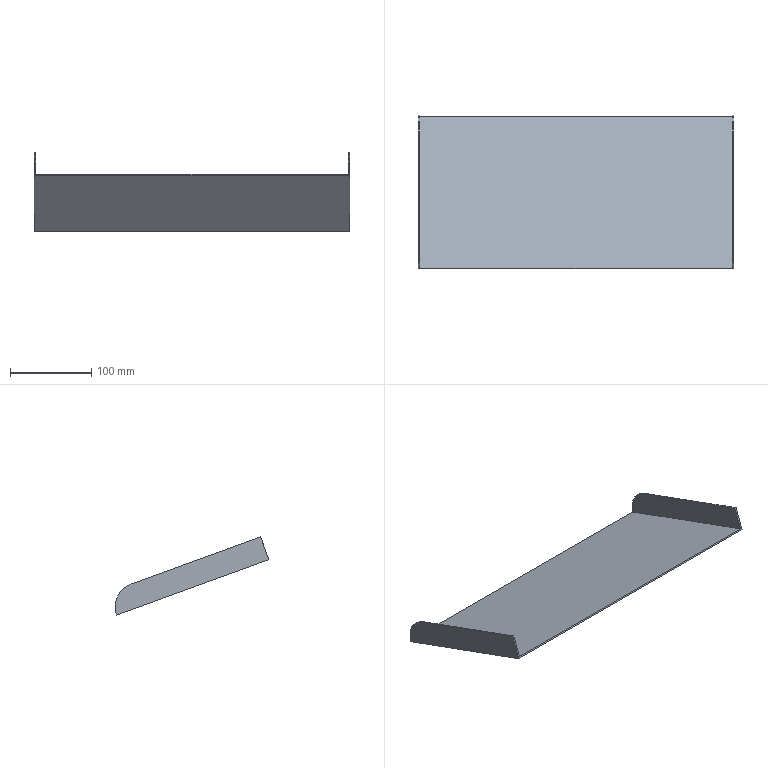Part | NX | features solid 2 | 1 solid | 12 faces | box 389.78 x 189.748 x 96.595 mm | volume 177540 mm3 | plane 10 | cylinder 2 | commonest cylinder face diameters 60 x2
STEP:
#1=CARTESIAN_POINT('',(397.22,1010.,-315.103));
#2=VERTEX_POINT('',#1);
#3=CARTESIAN_POINT('',(397.22,1197.876,-383.484));
#4=VERTEX_POINT('',#3);
#5=CARTESIAN_POINT('',(397.22,1038.191,-325.364));
#6=DIRECTION('',(0.,0.9397,-0.342));
#7=VECTOR('',#6,1000.);
#8=LINE('',#5,#7);
#9=EDGE_CURVE('',#2,#4,#8,.T.);
#10=ORIENTED_EDGE('',*,*,#9,.F.);
#11=CARTESIAN_POINT('',(783.,1010.,-315.103));
#12=VERTEX_POINT('',#11);
#13=CARTESIAN_POINT('',(407.22,1010.,-315.103));
#14=DIRECTION('',(-1.,0.,0.));
#15=VECTOR('',#14,1000.);
#16=LINE('',#13,#15);
#17=EDGE_CURVE('',#2,#12,#16,.F.);
#18=ORIENTED_EDGE('',*,*,#17,.T.);
#19=CARTESIAN_POINT('',(783.,1197.876,-383.484));
#20=VERTEX_POINT('',#19);
#21=CARTESIAN_POINT('',(783.,1038.191,-325.364));
#22=DIRECTION('',(0.,0.9397,-0.342));
#23=VECTOR('',#22,1000.);
#24=LINE('',#21,#23);
#25=EDGE_CURVE('',#12,#20,#24,.T.);
#26=ORIENTED_EDGE('',*,*,#25,.T.);
#27=CARTESIAN_POINT('',(785.,1197.876,-383.484));
#28=VERTEX_POINT('',#27);
#29=CARTESIAN_POINT('',(785.,1197.876,-383.484));
#30=CARTESIAN_POINT('',(784.333,1197.876,-383.484));
#31=CARTESIAN_POINT('',(783.667,1197.876,-383.484));
#32=CARTESIAN_POINT('',(783.,1197.876,-383.484));
#33=B_SPLINE_CURVE_WITH_KNOTS('',3,(#29,#30,#31,#32),.UNSPECIFIED.,.F.,.F.,(4,4),(1310.699,1310.701),.UNSPECIFIED.);
#34=EDGE_CURVE('',#28,#20,#33,.T.);
#35=ORIENTED_EDGE('',*,*,#34,.F.);
#36=CARTESIAN_POINT('',(785.,1197.939,-383.507));
#37=VERTEX_POINT('',#36);
#38=CARTESIAN_POINT('',(785.,1038.191,-325.364));
#39=DIRECTION('',(0.,-0.9397,0.342));
#40=VECTOR('',#39,1000.);
#41=LINE('',#38,#40);
#42=EDGE_CURVE('',#28,#37,#41,.F.);
#43=ORIENTED_EDGE('',*,*,#42,.T.);
#44=CARTESIAN_POINT('',(395.22,1197.939,-383.507));
#45=VERTEX_POINT('',#44);
#46=CARTESIAN_POINT('',(407.22,1197.939,-383.507));
#47=DIRECTION('',(1.,0.,0.));
#48=VECTOR('',#47,1000.);
#49=LINE('',#46,#48);
#50=EDGE_CURVE('',#45,#37,#49,.T.);
#51=ORIENTED_EDGE('',*,*,#50,.F.);
#52=CARTESIAN_POINT('',(395.22,1197.876,-383.484));
#53=VERTEX_POINT('',#52);
#54=CARTESIAN_POINT('',(395.22,1038.191,-325.364));
#55=DIRECTION('',(0.,0.9397,-0.342));
#56=VECTOR('',#55,1000.);
#57=LINE('',#54,#56);
#58=EDGE_CURVE('',#53,#45,#57,.T.);
#59=ORIENTED_EDGE('',*,*,#58,.F.);
#60=CARTESIAN_POINT('',(397.22,1197.876,-383.484));
#61=CARTESIAN_POINT('',(396.553,1197.876,-383.484));
#62=CARTESIAN_POINT('',(395.886,1197.876,-383.484));
#63=CARTESIAN_POINT('',(395.22,1197.876,-383.484));
#64=B_SPLINE_CURVE_WITH_KNOTS('',3,(#60,#61,#62,#63),.UNSPECIFIED.,.F.,.F.,(4,4),(1310.699,1310.701),.UNSPECIFIED.);
#65=EDGE_CURVE('',#4,#53,#64,.T.);
#66=ORIENTED_EDGE('',*,*,#65,.F.);
#67=EDGE_LOOP('',(#10,#18,#26,#35,#43,#51,#59,#66));
#68=FACE_BOUND('',#67,.T.);
#69=CARTESIAN_POINT('',(407.22,1038.191,-325.364));
#70=DIRECTION('',(0.,0.342,0.9397));
#71=DIRECTION('',(1.,0.,0.));
#72=AXIS2_PLACEMENT_3D('',#69,#70,#71);
#73=PLANE('',#72);
#74=ADVANCED_FACE('',(#68),#73,.T.);
#75=ORIENTED_EDGE('',*,*,#17,.F.);
#76=CARTESIAN_POINT('',(397.22,1019.577,-288.792));
#77=VERTEX_POINT('',#76);
#78=CARTESIAN_POINT('',(397.22,1009.316,-316.982));
#79=DIRECTION('',(0.,-0.342,-0.9397));
#80=VECTOR('',#79,1000.);
#81=LINE('',#78,#80);
#82=EDGE_CURVE('',#2,#77,#81,.F.);
#83=ORIENTED_EDGE('',*,*,#82,.T.);
#84=CARTESIAN_POINT('',(395.22,1019.577,-288.792));
#85=VERTEX_POINT('',#84);
#86=CARTESIAN_POINT('',(395.22,1019.577,-288.792));
#87=DIRECTION('',(1.,0.,0.));
#88=VECTOR('',#87,1000.);
#89=LINE('',#86,#88);
#90=EDGE_CURVE('',#85,#77,#89,.T.);
#91=ORIENTED_EDGE('',*,*,#90,.F.);
#92=CARTESIAN_POINT('',(395.22,1009.316,-316.982));
#93=VERTEX_POINT('',#92);
#94=CARTESIAN_POINT('',(395.22,1010.,-315.103));
#95=DIRECTION('',(0.,0.342,0.9397));
#96=VECTOR('',#95,1000.);
#97=LINE('',#94,#96);
#98=EDGE_CURVE('',#85,#93,#97,.F.);
#99=ORIENTED_EDGE('',*,*,#98,.T.);
#100=CARTESIAN_POINT('',(785.,1009.316,-316.982));
#101=VERTEX_POINT('',#100);
#102=CARTESIAN_POINT('',(407.22,1009.316,-316.982));
#103=DIRECTION('',(-1.,0.,0.));
#104=VECTOR('',#103,1000.);
#105=LINE('',#102,#104);
#106=EDGE_CURVE('',#93,#101,#105,.F.);
#107=ORIENTED_EDGE('',*,*,#106,.T.);
#108=CARTESIAN_POINT('',(785.,1019.577,-288.792));
#109=VERTEX_POINT('',#108);
#110=CARTESIAN_POINT('',(785.,1010.,-315.103));
#111=DIRECTION('',(0.,-0.342,-0.9397));
#112=VECTOR('',#111,1000.);
#113=LINE('',#110,#112);
#114=EDGE_CURVE('',#109,#101,#113,.T.);
#115=ORIENTED_EDGE('',*,*,#114,.F.);
#116=CARTESIAN_POINT('',(783.,1019.577,-288.792));
#117=VERTEX_POINT('',#116);
#118=CARTESIAN_POINT('',(785.,1019.577,-288.792));
#119=DIRECTION('',(1.,0.,0.));
#120=VECTOR('',#119,1000.);
#121=LINE('',#118,#120);
#122=EDGE_CURVE('',#109,#117,#121,.F.);
#123=ORIENTED_EDGE('',*,*,#122,.T.);
#124=CARTESIAN_POINT('',(783.,1009.316,-316.982));
#125=DIRECTION('',(0.,-0.342,-0.9397));
#126=VECTOR('',#125,1000.);
#127=LINE('',#124,#126);
#128=EDGE_CURVE('',#12,#117,#127,.F.);
#129=ORIENTED_EDGE('',*,*,#128,.F.);
#130=EDGE_LOOP('',(#75,#83,#91,#99,#107,#115,#123,#129));
#131=FACE_BOUND('',#130,.T.);
#132=CARTESIAN_POINT('',(407.22,1010.,-315.103));
#133=DIRECTION('',(0.,-0.9397,0.342));
#134=DIRECTION('',(1.,0.,0.));
#135=AXIS2_PLACEMENT_3D('',#132,#133,#134);
#136=PLANE('',#135);
#137=ADVANCED_FACE('',(#131),#136,.T.);
#138=ORIENTED_EDGE('',*,*,#42,.F.);
#139=CARTESIAN_POINT('',(785.,1179.324,-346.935));
#140=VERTEX_POINT('',#139);
#141=CARTESIAN_POINT('',(785.,1169.064,-375.126));
#142=DIRECTION('',(1.,0.,0.));
#143=DIRECTION('',(0.,-0.342,-0.9397));
#144=AXIS2_PLACEMENT_3D('',#141,#142,#143);
#145=CIRCLE('',#144,30.);
#146=EDGE_CURVE('',#28,#140,#145,.T.);
#147=ORIENTED_EDGE('',*,*,#146,.T.);
#148=CARTESIAN_POINT('',(785.,1019.577,-288.792));
#149=DIRECTION('',(0.,0.9397,-0.342));
#150=VECTOR('',#149,1000.);
#151=LINE('',#148,#150);
#152=EDGE_CURVE('',#109,#140,#151,.T.);
#153=ORIENTED_EDGE('',*,*,#152,.F.);
#154=ORIENTED_EDGE('',*,*,#114,.T.);
#155=CARTESIAN_POINT('',(785.,1197.254,-385.386));
#156=VERTEX_POINT('',#155);
#157=CARTESIAN_POINT('',(785.,1037.507,-327.243));
#158=DIRECTION('',(0.,-0.9397,0.342));
#159=VECTOR('',#158,1000.);
#160=LINE('',#157,#159);
#161=EDGE_CURVE('',#101,#156,#160,.F.);
#162=ORIENTED_EDGE('',*,*,#161,.T.);
#163=CARTESIAN_POINT('',(785.,1197.939,-383.507));
#164=DIRECTION('',(0.,0.342,0.9397));
#165=VECTOR('',#164,1000.);
#166=LINE('',#163,#165);
#167=EDGE_CURVE('',#37,#156,#166,.F.);
#168=ORIENTED_EDGE('',*,*,#167,.F.);
#169=EDGE_LOOP('',(#138,#147,#153,#154,#162,#168));
#170=FACE_BOUND('',#169,.T.);
#171=CARTESIAN_POINT('',(785.,1038.191,-325.364));
#172=DIRECTION('',(1.,0.,0.));
#173=DIRECTION('',(0.,0.9397,-0.342));
#174=AXIS2_PLACEMENT_3D('',#171,#172,#173);
#175=PLANE('',#174);
#176=ADVANCED_FACE('',(#170),#175,.T.);
#177=ORIENTED_EDGE('',*,*,#167,.T.);
#178=CARTESIAN_POINT('',(395.22,1197.254,-385.386));
#179=VERTEX_POINT('',#178);
#180=CARTESIAN_POINT('',(407.22,1197.254,-385.386));
#181=DIRECTION('',(1.,0.,0.));
#182=VECTOR('',#181,1000.);
#183=LINE('',#180,#182);
#184=EDGE_CURVE('',#179,#156,#183,.T.);
#185=ORIENTED_EDGE('',*,*,#184,.F.);
#186=CARTESIAN_POINT('',(395.22,1197.939,-383.507));
#187=DIRECTION('',(0.,-0.342,-0.9397));
#188=VECTOR('',#187,1000.);
#189=LINE('',#186,#188);
#190=EDGE_CURVE('',#45,#179,#189,.T.);
#191=ORIENTED_EDGE('',*,*,#190,.F.);
#192=ORIENTED_EDGE('',*,*,#50,.T.);
#193=EDGE_LOOP('',(#177,#185,#191,#192));
#194=FACE_BOUND('',#193,.T.);
#195=CARTESIAN_POINT('',(407.22,1197.939,-383.507));
#196=DIRECTION('',(0.,-0.9397,0.342));
#197=DIRECTION('',(1.,0.,0.));
#198=AXIS2_PLACEMENT_3D('',#195,#196,#197);
#199=PLANE('',#198);
#200=ADVANCED_FACE('',(#194),#199,.F.);
#201=ORIENTED_EDGE('',*,*,#190,.T.);
#202=CARTESIAN_POINT('',(395.22,1037.507,-327.243));
#203=DIRECTION('',(0.,0.9397,-0.342));
#204=VECTOR('',#203,1000.);
#205=LINE('',#202,#204);
#206=EDGE_CURVE('',#93,#179,#205,.T.);
#207=ORIENTED_EDGE('',*,*,#206,.F.);
#208=ORIENTED_EDGE('',*,*,#98,.F.);
#209=CARTESIAN_POINT('',(395.22,1179.324,-346.935));
#210=VERTEX_POINT('',#209);
#211=CARTESIAN_POINT('',(395.22,1019.577,-288.792));
#212=DIRECTION('',(0.,0.9397,-0.342));
#213=VECTOR('',#212,1000.);
#214=LINE('',#211,#213);
#215=EDGE_CURVE('',#85,#210,#214,.T.);
#216=ORIENTED_EDGE('',*,*,#215,.T.);
#217=CARTESIAN_POINT('',(395.22,1169.064,-375.126));
#218=DIRECTION('',(1.,0.,0.));
#219=DIRECTION('',(0.,-0.342,-0.9397));
#220=AXIS2_PLACEMENT_3D('',#217,#218,#219);
#221=CIRCLE('',#220,30.);
#222=EDGE_CURVE('',#210,#53,#221,.F.);
#223=ORIENTED_EDGE('',*,*,#222,.T.);
#224=ORIENTED_EDGE('',*,*,#58,.T.);
#225=EDGE_LOOP('',(#201,#207,#208,#216,#223,#224));
#226=FACE_BOUND('',#225,.T.);
#227=CARTESIAN_POINT('',(395.22,1038.191,-325.364));
#228=DIRECTION('',(1.,0.,0.));
#229=DIRECTION('',(0.,0.9397,-0.342));
#230=AXIS2_PLACEMENT_3D('',#227,#228,#229);
#231=PLANE('',#230);
#232=ADVANCED_FACE('',(#226),#231,.F.);
#233=ORIENTED_EDGE('',*,*,#161,.F.);
#234=ORIENTED_EDGE('',*,*,#106,.F.);
#235=ORIENTED_EDGE('',*,*,#206,.T.);
#236=ORIENTED_EDGE('',*,*,#184,.T.);
#237=EDGE_LOOP('',(#233,#234,#235,#236));
#238=FACE_BOUND('',#237,.T.);
#239=CARTESIAN_POINT('',(407.22,1037.507,-327.243));
#240=DIRECTION('',(0.,0.342,0.9397));
#241=DIRECTION('',(1.,0.,0.));
#242=AXIS2_PLACEMENT_3D('',#239,#240,#241);
#243=PLANE('',#242);
#244=ADVANCED_FACE('',(#238),#243,.F.);
#245=ORIENTED_EDGE('',*,*,#152,.T.);
#246=CARTESIAN_POINT('',(783.,1179.324,-346.935));
#247=VERTEX_POINT('',#246);
#248=CARTESIAN_POINT('',(785.,1179.324,-346.935));
#249=DIRECTION('',(1.,0.,0.));
#250=VECTOR('',#249,1000.);
#251=LINE('',#248,#250);
#252=EDGE_CURVE('',#140,#247,#251,.F.);
#253=ORIENTED_EDGE('',*,*,#252,.T.);
#254=CARTESIAN_POINT('',(783.,1019.577,-288.792));
#255=DIRECTION('',(0.,0.9397,-0.342));
#256=VECTOR('',#255,1000.);
#257=LINE('',#254,#256);
#258=EDGE_CURVE('',#117,#247,#257,.T.);
#259=ORIENTED_EDGE('',*,*,#258,.F.);
#260=ORIENTED_EDGE('',*,*,#122,.F.);
#261=EDGE_LOOP('',(#245,#253,#259,#260));
#262=FACE_BOUND('',#261,.T.);
#263=CARTESIAN_POINT('',(785.,1019.577,-288.792));
#264=DIRECTION('',(0.,-0.342,-0.9397));
#265=DIRECTION('',(0.,0.9397,-0.342));
#266=AXIS2_PLACEMENT_3D('',#263,#264,#265);
#267=PLANE('',#266);
#268=ADVANCED_FACE('',(#262),#267,.F.);
#269=ORIENTED_EDGE('',*,*,#25,.F.);
#270=ORIENTED_EDGE('',*,*,#128,.T.);
#271=ORIENTED_EDGE('',*,*,#258,.T.);
#272=CARTESIAN_POINT('',(783.,1169.064,-375.126));
#273=DIRECTION('',(1.,0.,0.));
#274=DIRECTION('',(0.,-0.342,-0.9397));
#275=AXIS2_PLACEMENT_3D('',#272,#273,#274);
#276=CIRCLE('',#275,30.);
#277=EDGE_CURVE('',#247,#20,#276,.F.);
#278=ORIENTED_EDGE('',*,*,#277,.T.);
#279=EDGE_LOOP('',(#269,#270,#271,#278));
#280=FACE_BOUND('',#279,.T.);
#281=CARTESIAN_POINT('',(783.,1009.316,-316.982));
#282=DIRECTION('',(1.,0.,0.));
#283=DIRECTION('',(0.,-0.342,-0.9397));
#284=AXIS2_PLACEMENT_3D('',#281,#282,#283);
#285=PLANE('',#284);
#286=ADVANCED_FACE('',(#280),#285,.F.);
#287=ORIENTED_EDGE('',*,*,#146,.F.);
#288=ORIENTED_EDGE('',*,*,#34,.T.);
#289=ORIENTED_EDGE('',*,*,#277,.F.);
#290=ORIENTED_EDGE('',*,*,#252,.F.);
#291=EDGE_LOOP('',(#287,#288,#289,#290));
#292=FACE_BOUND('',#291,.T.);
#293=CARTESIAN_POINT('',(785.,1169.064,-375.126));
#294=DIRECTION('',(1.,0.,0.));
#295=DIRECTION('',(0.,-0.342,-0.9397));
#296=AXIS2_PLACEMENT_3D('',#293,#294,#295);
#297=CYLINDRICAL_SURFACE('',#296,30.);
#298=ADVANCED_FACE('',(#292),#297,.T.);
#299=CARTESIAN_POINT('',(397.22,1179.324,-346.935));
#300=VERTEX_POINT('',#299);
#301=CARTESIAN_POINT('',(397.22,1019.577,-288.792));
#302=DIRECTION('',(0.,0.9397,-0.342));
#303=VECTOR('',#302,1000.);
#304=LINE('',#301,#303);
#305=EDGE_CURVE('',#77,#300,#304,.T.);
#306=ORIENTED_EDGE('',*,*,#305,.T.);
#307=CARTESIAN_POINT('',(395.22,1179.324,-346.935));
#308=DIRECTION('',(1.,0.,0.));
#309=VECTOR('',#308,1000.);
#310=LINE('',#307,#309);
#311=EDGE_CURVE('',#300,#210,#310,.F.);
#312=ORIENTED_EDGE('',*,*,#311,.T.);
#313=ORIENTED_EDGE('',*,*,#215,.F.);
#314=ORIENTED_EDGE('',*,*,#90,.T.);
#315=EDGE_LOOP('',(#306,#312,#313,#314));
#316=FACE_BOUND('',#315,.T.);
#317=CARTESIAN_POINT('',(395.22,1019.577,-288.792));
#318=DIRECTION('',(0.,-0.342,-0.9397));
#319=DIRECTION('',(0.,0.9397,-0.342));
#320=AXIS2_PLACEMENT_3D('',#317,#318,#319);
#321=PLANE('',#320);
#322=ADVANCED_FACE('',(#316),#321,.F.);
#323=ORIENTED_EDGE('',*,*,#82,.F.);
#324=ORIENTED_EDGE('',*,*,#9,.T.);
#325=CARTESIAN_POINT('',(397.22,1169.064,-375.126));
#326=DIRECTION('',(1.,0.,0.));
#327=DIRECTION('',(0.,-0.342,-0.9397));
#328=AXIS2_PLACEMENT_3D('',#325,#326,#327);
#329=CIRCLE('',#328,30.);
#330=EDGE_CURVE('',#4,#300,#329,.T.);
#331=ORIENTED_EDGE('',*,*,#330,.T.);
#332=ORIENTED_EDGE('',*,*,#305,.F.);
#333=EDGE_LOOP('',(#323,#324,#331,#332));
#334=FACE_BOUND('',#333,.T.);
#335=CARTESIAN_POINT('',(397.22,1009.316,-316.982));
#336=DIRECTION('',(1.,0.,0.));
#337=DIRECTION('',(0.,-0.342,-0.9397));
#338=AXIS2_PLACEMENT_3D('',#335,#336,#337);
#339=PLANE('',#338);
#340=ADVANCED_FACE('',(#334),#339,.T.);
#341=ORIENTED_EDGE('',*,*,#330,.F.);
#342=ORIENTED_EDGE('',*,*,#65,.T.);
#343=ORIENTED_EDGE('',*,*,#222,.F.);
#344=ORIENTED_EDGE('',*,*,#311,.F.);
#345=EDGE_LOOP('',(#341,#342,#343,#344));
#346=FACE_BOUND('',#345,.T.);
#347=CARTESIAN_POINT('',(395.22,1169.064,-375.126));
#348=DIRECTION('',(-1.,0.,0.));
#349=DIRECTION('',(0.,0.342,0.9397));
#350=AXIS2_PLACEMENT_3D('',#347,#348,#349);
#351=CYLINDRICAL_SURFACE('',#350,30.);
#352=ADVANCED_FACE('',(#346),#351,.T.);
#353=CLOSED_SHELL('',(#74,#137,#176,#200,#232,#244,#268,#286,#298,#322,#340,#352));
#354=MANIFOLD_SOLID_BREP('',#353);
#355=(LENGTH_UNIT()NAMED_UNIT(*)SI_UNIT(.MILLI.,.METRE.));
#356=UNCERTAINTY_MEASURE_WITH_UNIT(LENGTH_MEASURE(0.0508),#355,'','');
#357=(NAMED_UNIT(*)PLANE_ANGLE_UNIT()SI_UNIT($,.RADIAN.));
#358=(NAMED_UNIT(*)SI_UNIT($,.STERADIAN.)SOLID_ANGLE_UNIT());
#359=(GEOMETRIC_REPRESENTATION_CONTEXT(3)GLOBAL_UNCERTAINTY_ASSIGNED_CONTEXT((#356))GLOBAL_UNIT_ASSIGNED_CONTEXT((#355,#357,#358))REPRESENTATION_CONTEXT('',''));
#360=ADVANCED_BREP_SHAPE_REPRESENTATION('',(#354),#359);